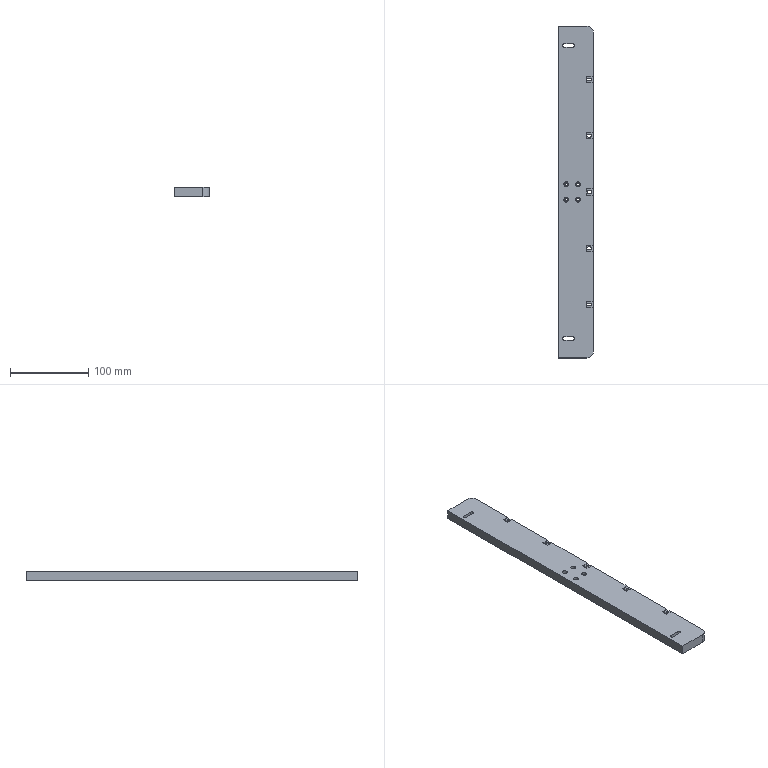Part | SolidWorks | features ICE 5, Extrusion 1, Fillet 1, HoleWzd 1, LPattern 1 | 1 solid | 125 faces | box 44 x 425 x 12 mm | volume 219009 mm3 | plane 65 | cylinder 60 | commonest cylinder face diameters 6 x23 3.2 x15 3.4 x8 4 x6 8 x6 16 x2